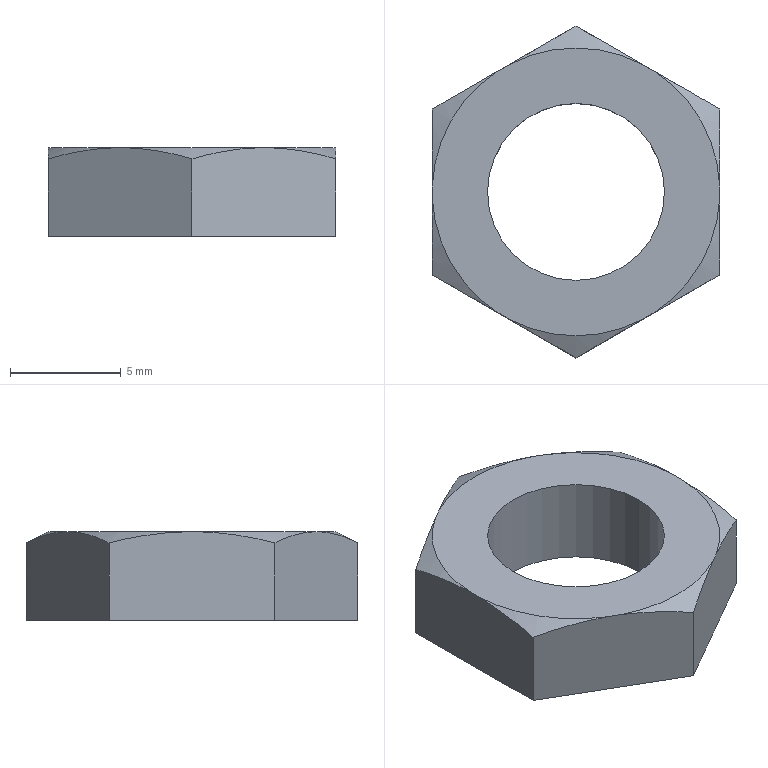Part | STEP file | E2B_S08KS01_WP_C1_CLAMPING_NUT | 1 solid | 16 faces | box 13 x 15.011 x 4 mm | volume 382.328 mm3 | plane 8 | cone 6 | cylinder 2 | commonest cylinder face diameters 8 x2